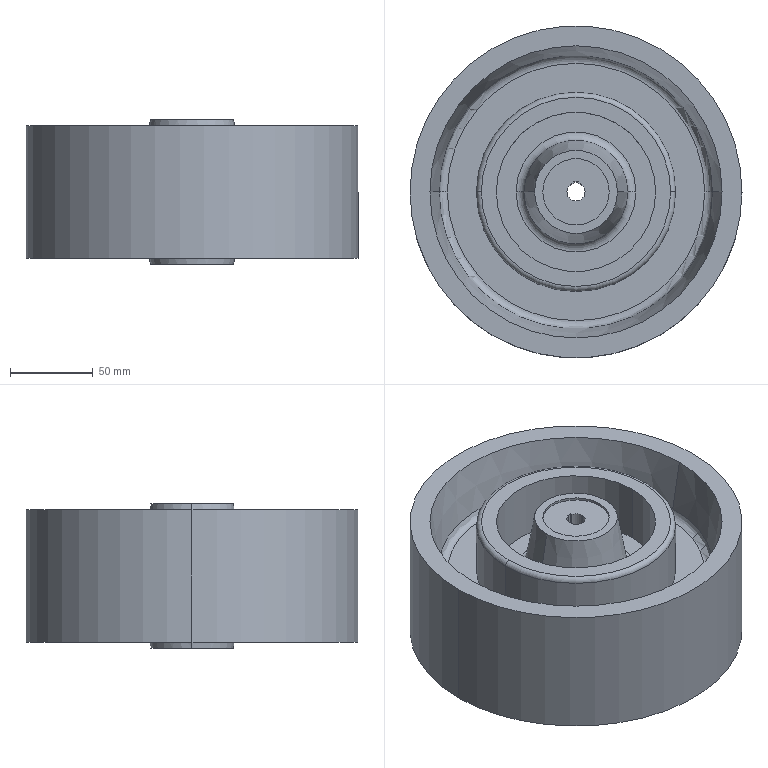Part | SolidWorks | features ICE 3, Fillet 2, Extrusion 1, Revolution 1 | 1 solid | 68 faces | box 200 x 200 x 87 mm | volume 1384967 mm3 | plane 31 | cylinder 17 | torus 12 | cone 8 | commonest cylinder face diameters 40 x4 96 x4 120 x4 11 x3 200 x2